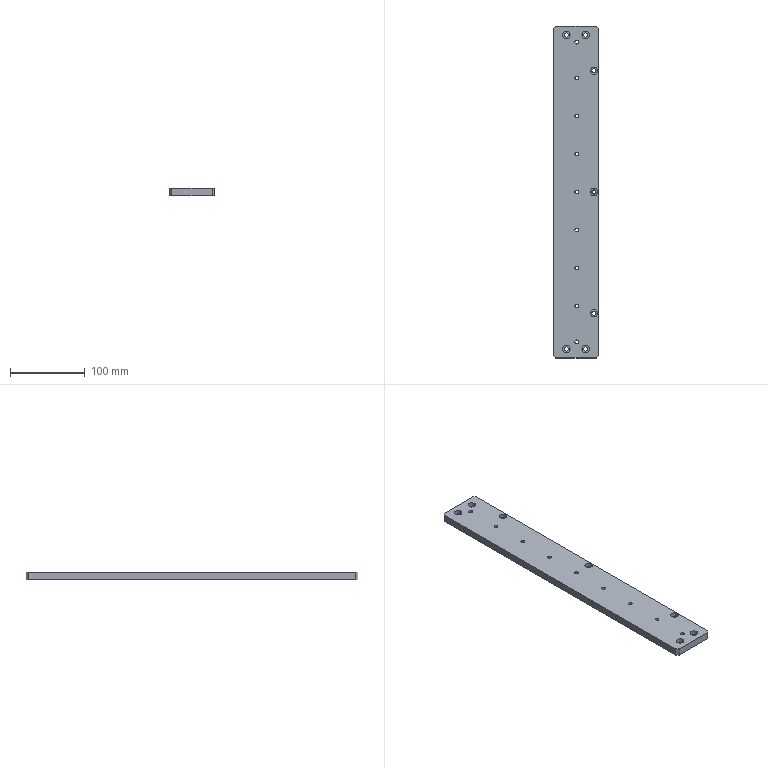Part | STEP file | PN_0007 | 1 solid | 63 faces | box 60 x 444 x 10 mm | volume 260719 mm3 | cylinder 46 | plane 17 | commonest cylinder face diameters 5 x18 5.5 x14 10 x14